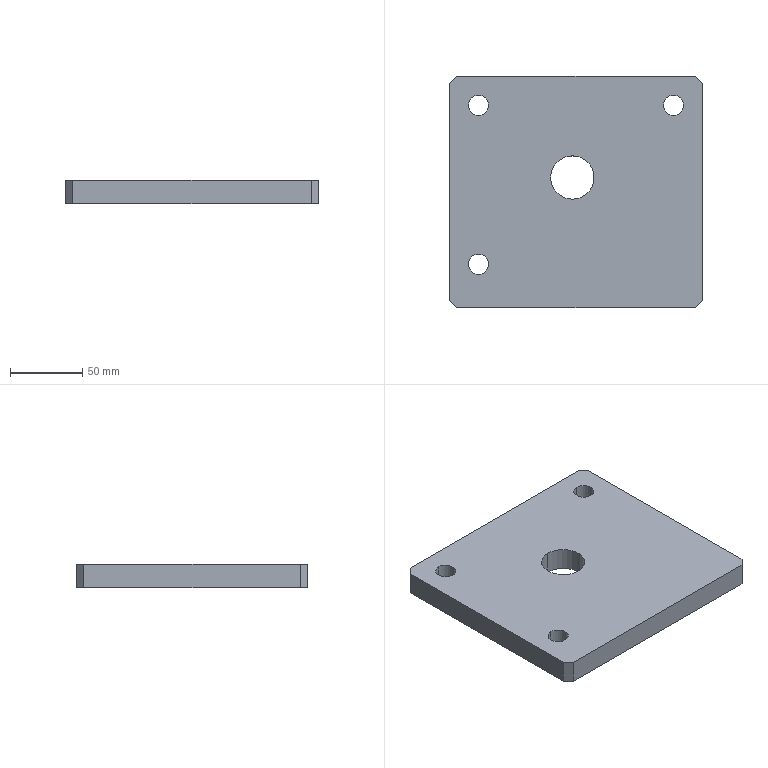Part | STEP file | [03]-5 | 1 solid | 18 faces | box 175 x 160 x 16 mm | volume 428501 mm3 | plane 10 | cylinder 8 | commonest cylinder face diameters 14 x6 30 x2